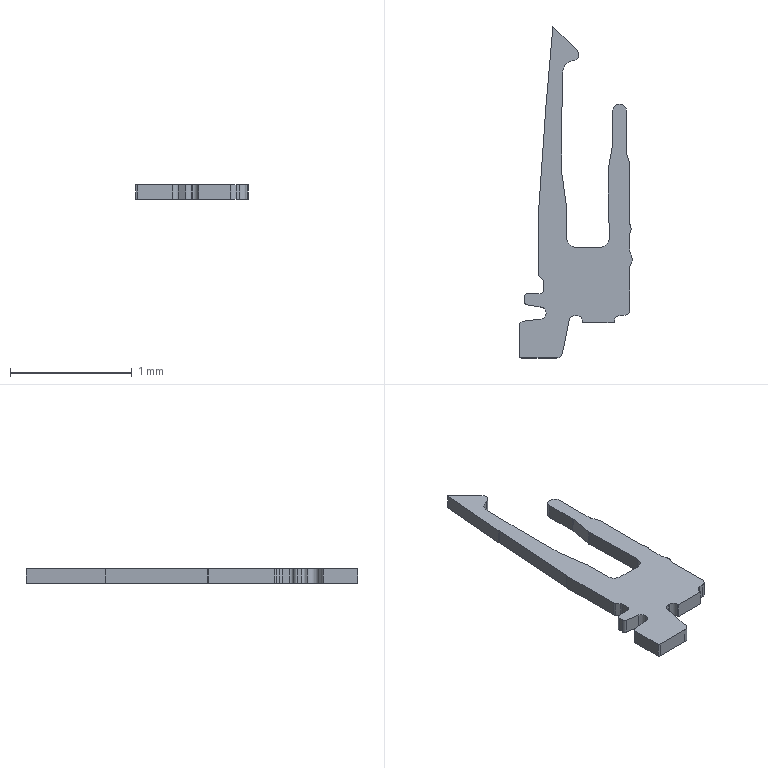Part | Creo | 1 solid | 71 faces | box 0.9275 x 2.732 x 0.12 mm | volume 0.1258 mm3 | plane 40 | cylinder 31 | commonest cylinder face diameters 0.1 x21 0.06 x5 0.2 x3 0.16 x2